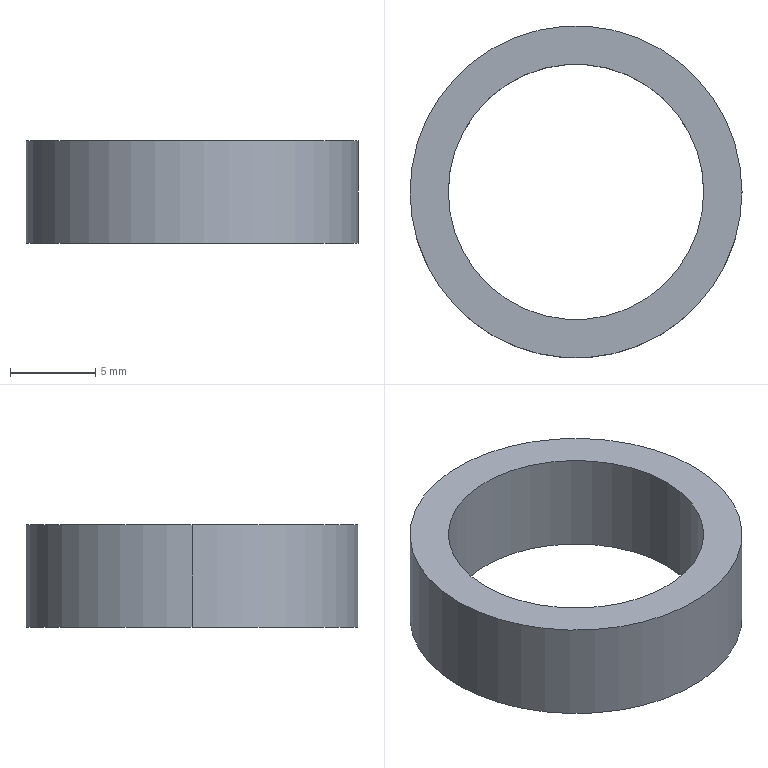Part | SolidWorks | features BaseBody 1 | 1 solid | 6 faces | box 19.5 x 19.5 x 6 mm | volume 731.598 mm3 | cylinder 4 | plane 2 | commonest cylinder face diameters 15 x2 19.5 x2
STEP:
#1=CARTESIAN_POINT('',(-137.246,1831.544,-1.5));
#2=VERTEX_POINT('',#1);
#3=CARTESIAN_POINT('',(-117.746,1831.544,-1.5));
#4=VERTEX_POINT('',#3);
#5=CARTESIAN_POINT('',(-127.496,1831.544,-1.5));
#6=DIRECTION('',(0.,0.,-1.));
#7=DIRECTION('',(-1.,0.,0.));
#8=AXIS2_PLACEMENT_3D('',#5,#6,#7);
#9=CIRCLE('',#8,9.75);
#10=EDGE_CURVE('',#2,#4,#9,.T.);
#11=ORIENTED_EDGE('',*,*,#10,.T.);
#12=CARTESIAN_POINT('',(-117.746,1831.544,-7.5));
#13=VERTEX_POINT('',#12);
#14=CARTESIAN_POINT('',(-117.746,1831.544,-1.5));
#15=DIRECTION('',(0.,0.,-1.));
#16=VECTOR('',#15,1000.);
#17=LINE('',#14,#16);
#18=EDGE_CURVE('',#4,#13,#17,.T.);
#19=ORIENTED_EDGE('',*,*,#18,.T.);
#20=CARTESIAN_POINT('',(-137.246,1831.544,-7.5));
#21=VERTEX_POINT('',#20);
#22=CARTESIAN_POINT('',(-127.496,1831.544,-7.5));
#23=DIRECTION('',(0.,0.,1.));
#24=DIRECTION('',(-1.,0.,0.));
#25=AXIS2_PLACEMENT_3D('',#22,#23,#24);
#26=CIRCLE('',#25,9.75);
#27=EDGE_CURVE('',#13,#21,#26,.T.);
#28=ORIENTED_EDGE('',*,*,#27,.T.);
#29=CARTESIAN_POINT('',(-137.246,1831.544,-1.5));
#30=DIRECTION('',(0.,0.,-1.));
#31=VECTOR('',#30,1000.);
#32=LINE('',#29,#31);
#33=EDGE_CURVE('',#2,#21,#32,.T.);
#34=ORIENTED_EDGE('',*,*,#33,.F.);
#35=EDGE_LOOP('',(#11,#19,#28,#34));
#36=FACE_OUTER_BOUND('',#35,.T.);
#37=CARTESIAN_POINT('',(-127.496,1831.544,-1.5));
#38=DIRECTION('',(0.,0.,-1.));
#39=DIRECTION('',(-1.,0.,0.));
#40=AXIS2_PLACEMENT_3D('',#37,#38,#39);
#41=CYLINDRICAL_SURFACE('',#40,9.75);
#42=ADVANCED_FACE('',(#36),#41,.T.);
#43=CARTESIAN_POINT('',(-119.996,1831.544,-1.5));
#44=VERTEX_POINT('',#43);
#45=CARTESIAN_POINT('',(-134.996,1831.544,-1.5));
#46=VERTEX_POINT('',#45);
#47=CARTESIAN_POINT('',(-127.496,1831.544,-1.5));
#48=DIRECTION('',(0.,0.,-1.));
#49=DIRECTION('',(-1.,0.,0.));
#50=AXIS2_PLACEMENT_3D('',#47,#48,#49);
#51=CIRCLE('',#50,7.5);
#52=EDGE_CURVE('',#44,#46,#51,.T.);
#53=ORIENTED_EDGE('',*,*,#52,.F.);
#54=CARTESIAN_POINT('',(-119.996,1831.544,-7.5));
#55=VERTEX_POINT('',#54);
#56=CARTESIAN_POINT('',(-119.996,1831.544,-1.5));
#57=DIRECTION('',(0.,0.,-1.));
#58=VECTOR('',#57,1000.);
#59=LINE('',#56,#58);
#60=EDGE_CURVE('',#44,#55,#59,.T.);
#61=ORIENTED_EDGE('',*,*,#60,.T.);
#62=CARTESIAN_POINT('',(-134.996,1831.544,-7.5));
#63=VERTEX_POINT('',#62);
#64=CARTESIAN_POINT('',(-127.496,1831.544,-7.5));
#65=DIRECTION('',(0.,0.,-1.));
#66=DIRECTION('',(-1.,0.,0.));
#67=AXIS2_PLACEMENT_3D('',#64,#65,#66);
#68=CIRCLE('',#67,7.5);
#69=EDGE_CURVE('',#55,#63,#68,.T.);
#70=ORIENTED_EDGE('',*,*,#69,.T.);
#71=CARTESIAN_POINT('',(-134.996,1831.544,-1.5));
#72=DIRECTION('',(0.,0.,-1.));
#73=VECTOR('',#72,1000.);
#74=LINE('',#71,#73);
#75=EDGE_CURVE('',#46,#63,#74,.T.);
#76=ORIENTED_EDGE('',*,*,#75,.F.);
#77=EDGE_LOOP('',(#53,#61,#70,#76));
#78=FACE_OUTER_BOUND('',#77,.T.);
#79=CARTESIAN_POINT('',(-127.496,1831.544,-1.5));
#80=DIRECTION('',(0.,0.,-1.));
#81=DIRECTION('',(-1.,0.,0.));
#82=AXIS2_PLACEMENT_3D('',#79,#80,#81);
#83=CYLINDRICAL_SURFACE('',#82,7.5);
#84=ADVANCED_FACE('',(#78),#83,.F.);
#85=ORIENTED_EDGE('',*,*,#18,.F.);
#86=CARTESIAN_POINT('',(-127.496,1831.544,-1.5));
#87=DIRECTION('',(0.,0.,-1.));
#88=DIRECTION('',(-1.,0.,0.));
#89=AXIS2_PLACEMENT_3D('',#86,#87,#88);
#90=CIRCLE('',#89,9.75);
#91=EDGE_CURVE('',#4,#2,#90,.T.);
#92=ORIENTED_EDGE('',*,*,#91,.T.);
#93=ORIENTED_EDGE('',*,*,#33,.T.);
#94=CARTESIAN_POINT('',(-127.496,1831.544,-7.5));
#95=DIRECTION('',(0.,0.,1.));
#96=DIRECTION('',(-1.,0.,0.));
#97=AXIS2_PLACEMENT_3D('',#94,#95,#96);
#98=CIRCLE('',#97,9.75);
#99=EDGE_CURVE('',#21,#13,#98,.T.);
#100=ORIENTED_EDGE('',*,*,#99,.T.);
#101=EDGE_LOOP('',(#85,#92,#93,#100));
#102=FACE_OUTER_BOUND('',#101,.T.);
#103=CARTESIAN_POINT('',(-127.496,1831.544,-1.5));
#104=DIRECTION('',(0.,0.,-1.));
#105=DIRECTION('',(-1.,0.,0.));
#106=AXIS2_PLACEMENT_3D('',#103,#104,#105);
#107=CYLINDRICAL_SURFACE('',#106,9.75);
#108=ADVANCED_FACE('',(#102),#107,.T.);
#109=CARTESIAN_POINT('',(-127.496,1831.544,-1.5));
#110=DIRECTION('',(0.,0.,-1.));
#111=DIRECTION('',(-1.,0.,0.));
#112=AXIS2_PLACEMENT_3D('',#109,#110,#111);
#113=CIRCLE('',#112,7.5);
#114=EDGE_CURVE('',#46,#44,#113,.T.);
#115=ORIENTED_EDGE('',*,*,#114,.T.);
#116=ORIENTED_EDGE('',*,*,#52,.T.);
#117=EDGE_LOOP('',(#115,#116));
#118=FACE_BOUND('',#117,.T.);
#119=ORIENTED_EDGE('',*,*,#10,.F.);
#120=ORIENTED_EDGE('',*,*,#91,.F.);
#121=EDGE_LOOP('',(#119,#120));
#122=FACE_OUTER_BOUND('',#121,.T.);
#123=CARTESIAN_POINT('',(-127.496,1831.544,-1.5));
#124=DIRECTION('',(0.,0.,1.));
#125=DIRECTION('',(1.,0.,0.));
#126=AXIS2_PLACEMENT_3D('',#123,#124,#125);
#127=PLANE('',#126);
#128=ADVANCED_FACE('',(#118,#122),#127,.T.);
#129=CARTESIAN_POINT('',(-127.496,1831.544,-7.5));
#130=DIRECTION('',(0.,0.,-1.));
#131=DIRECTION('',(-1.,0.,0.));
#132=AXIS2_PLACEMENT_3D('',#129,#130,#131);
#133=CIRCLE('',#132,7.5);
#134=EDGE_CURVE('',#63,#55,#133,.T.);
#135=ORIENTED_EDGE('',*,*,#134,.F.);
#136=ORIENTED_EDGE('',*,*,#69,.F.);
#137=EDGE_LOOP('',(#135,#136));
#138=FACE_BOUND('',#137,.T.);
#139=ORIENTED_EDGE('',*,*,#99,.F.);
#140=ORIENTED_EDGE('',*,*,#27,.F.);
#141=EDGE_LOOP('',(#139,#140));
#142=FACE_OUTER_BOUND('',#141,.T.);
#143=CARTESIAN_POINT('',(-127.496,1831.544,-7.5));
#144=DIRECTION('',(0.,0.,1.));
#145=DIRECTION('',(1.,0.,0.));
#146=AXIS2_PLACEMENT_3D('',#143,#144,#145);
#147=PLANE('',#146);
#148=ADVANCED_FACE('',(#138,#142),#147,.F.);
#149=ORIENTED_EDGE('',*,*,#60,.F.);
#150=ORIENTED_EDGE('',*,*,#114,.F.);
#151=ORIENTED_EDGE('',*,*,#75,.T.);
#152=ORIENTED_EDGE('',*,*,#134,.T.);
#153=EDGE_LOOP('',(#149,#150,#151,#152));
#154=FACE_OUTER_BOUND('',#153,.T.);
#155=CARTESIAN_POINT('',(-127.496,1831.544,-1.5));
#156=DIRECTION('',(0.,0.,-1.));
#157=DIRECTION('',(-1.,0.,0.));
#158=AXIS2_PLACEMENT_3D('',#155,#156,#157);
#159=CYLINDRICAL_SURFACE('',#158,7.5);
#160=ADVANCED_FACE('',(#154),#159,.F.);
#161=CLOSED_SHELL('',(#42,#84,#108,#128,#148,#160));
#162=MANIFOLD_SOLID_BREP('',#161);
#163=CARTESIAN_POINT('',(0.,0.,0.));
#164=DIRECTION('',(0.,0.,1.));
#165=DIRECTION('',(1.,0.,0.));
#166=AXIS2_PLACEMENT_3D('',#163,#164,#165);
#167=(LENGTH_UNIT()NAMED_UNIT(*)SI_UNIT(.MILLI.,.METRE.));
#168=UNCERTAINTY_MEASURE_WITH_UNIT(LENGTH_MEASURE(0.00001),#167,'','');
#169=(NAMED_UNIT(*)PLANE_ANGLE_UNIT()SI_UNIT($,.RADIAN.));
#170=(NAMED_UNIT(*)SI_UNIT($,.STERADIAN.)SOLID_ANGLE_UNIT());
#171=(GEOMETRIC_REPRESENTATION_CONTEXT(3)GLOBAL_UNCERTAINTY_ASSIGNED_CONTEXT((#168))GLOBAL_UNIT_ASSIGNED_CONTEXT((#167,#169,#170))REPRESENTATION_CONTEXT('',''));
#172=ADVANCED_BREP_SHAPE_REPRESENTATION('',(#162,#166),#171);